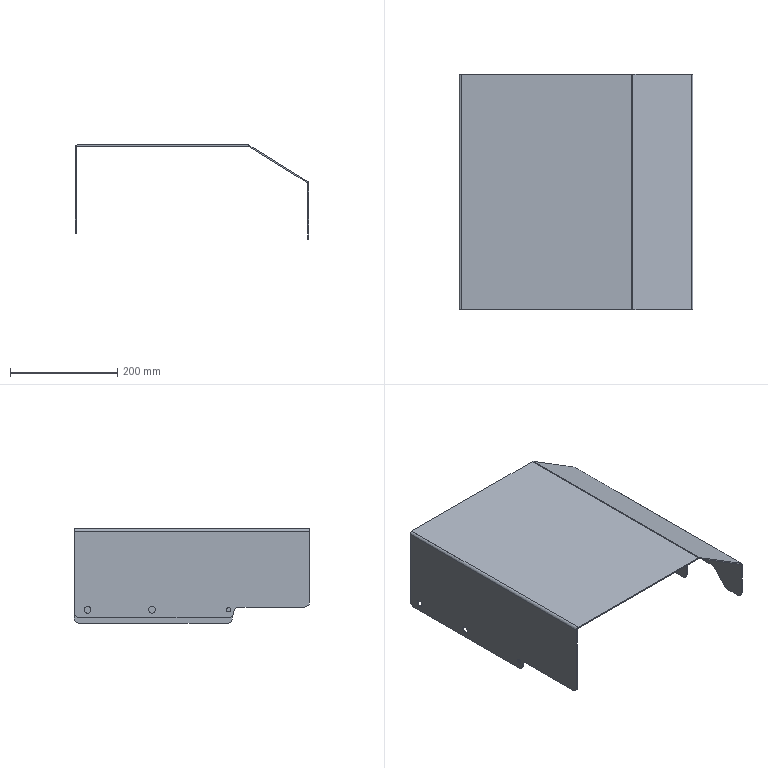Part | SolidWorks | features ICE 2, Fillet 1, FlatPattern 1, SMBaseFlange 1, SheetMetal 1 | 1 solid | 53 faces | box 436 x 439 x 176 mm | volume 705533 mm3 | plane 30 | cylinder 23 | commonest cylinder face diameters 20 x11 12.5 x4 5 x3 9.6 x3 8 x2
STEP:
#1=CARTESIAN_POINT('',(2.3,194.5,8.75));
#2=VERTEX_POINT('',#1);
#3=CARTESIAN_POINT('',(2.3,194.5,21.25));
#4=VERTEX_POINT('',#3);
#5=CARTESIAN_POINT('',(2.3,194.5,15.));
#6=DIRECTION('',(-1.,0.,0.));
#7=DIRECTION('',(0.,0.,-1.));
#8=AXIS2_PLACEMENT_3D('',#5,#6,#7);
#9=CIRCLE('',#8,6.25);
#10=EDGE_CURVE('',#2,#4,#9,.T.);
#11=ORIENTED_EDGE('',*,*,#10,.F.);
#12=CARTESIAN_POINT('',(0.,194.5,8.75));
#13=VERTEX_POINT('',#12);
#14=CARTESIAN_POINT('',(436.001,194.5,8.75));
#15=DIRECTION('',(-1.,0.,0.));
#16=VECTOR('',#15,1000.);
#17=LINE('',#14,#16);
#18=EDGE_CURVE('',#2,#13,#17,.T.);
#19=ORIENTED_EDGE('',*,*,#18,.T.);
#20=CARTESIAN_POINT('',(0.,194.5,21.25));
#21=VERTEX_POINT('',#20);
#22=CARTESIAN_POINT('',(0.,194.5,15.));
#23=DIRECTION('',(-1.,0.,0.));
#24=DIRECTION('',(0.,0.,1.));
#25=AXIS2_PLACEMENT_3D('',#22,#23,#24);
#26=CIRCLE('',#25,6.25);
#27=EDGE_CURVE('',#13,#21,#26,.T.);
#28=ORIENTED_EDGE('',*,*,#27,.T.);
#29=CARTESIAN_POINT('',(436.001,194.5,21.25));
#30=DIRECTION('',(-1.,0.,0.));
#31=VECTOR('',#30,1000.);
#32=LINE('',#29,#31);
#33=EDGE_CURVE('',#4,#21,#32,.T.);
#34=ORIENTED_EDGE('',*,*,#33,.F.);
#35=EDGE_LOOP('',(#11,#19,#28,#34));
#36=FACE_OUTER_BOUND('',#35,.T.);
#37=CARTESIAN_POINT('',(436.001,194.5,15.));
#38=DIRECTION('',(-1.,0.,0.));
#39=DIRECTION('',(0.,0.,1.));
#40=AXIS2_PLACEMENT_3D('',#37,#38,#39);
#41=CYLINDRICAL_SURFACE('',#40,6.25);
#42=ADVANCED_FACE('',(#36),#41,.F.);
#43=CARTESIAN_POINT('',(2.3,74.5,8.75));
#44=VERTEX_POINT('',#43);
#45=CARTESIAN_POINT('',(2.3,74.5,21.25));
#46=VERTEX_POINT('',#45);
#47=CARTESIAN_POINT('',(2.3,74.5,15.));
#48=DIRECTION('',(-1.,0.,0.));
#49=DIRECTION('',(0.,0.,-1.));
#50=AXIS2_PLACEMENT_3D('',#47,#48,#49);
#51=CIRCLE('',#50,6.25);
#52=EDGE_CURVE('',#44,#46,#51,.T.);
#53=ORIENTED_EDGE('',*,*,#52,.F.);
#54=CARTESIAN_POINT('',(0.,74.5,8.75));
#55=VERTEX_POINT('',#54);
#56=CARTESIAN_POINT('',(436.001,74.5,8.75));
#57=DIRECTION('',(-1.,0.,0.));
#58=VECTOR('',#57,1000.);
#59=LINE('',#56,#58);
#60=EDGE_CURVE('',#44,#55,#59,.T.);
#61=ORIENTED_EDGE('',*,*,#60,.T.);
#62=CARTESIAN_POINT('',(0.,74.5,21.25));
#63=VERTEX_POINT('',#62);
#64=CARTESIAN_POINT('',(0.,74.5,15.));
#65=DIRECTION('',(-1.,0.,0.));
#66=DIRECTION('',(0.,0.,1.));
#67=AXIS2_PLACEMENT_3D('',#64,#65,#66);
#68=CIRCLE('',#67,6.25);
#69=EDGE_CURVE('',#55,#63,#68,.T.);
#70=ORIENTED_EDGE('',*,*,#69,.T.);
#71=CARTESIAN_POINT('',(436.001,74.5,21.25));
#72=DIRECTION('',(-1.,0.,0.));
#73=VECTOR('',#72,1000.);
#74=LINE('',#71,#73);
#75=EDGE_CURVE('',#46,#63,#74,.T.);
#76=ORIENTED_EDGE('',*,*,#75,.F.);
#77=EDGE_LOOP('',(#53,#61,#70,#76));
#78=FACE_OUTER_BOUND('',#77,.T.);
#79=CARTESIAN_POINT('',(436.001,74.5,15.));
#80=DIRECTION('',(-1.,0.,0.));
#81=DIRECTION('',(0.,0.,1.));
#82=AXIS2_PLACEMENT_3D('',#79,#80,#81);
#83=CYLINDRICAL_SURFACE('',#82,6.25);
#84=ADVANCED_FACE('',(#78),#83,.F.);
#85=CARTESIAN_POINT('',(2.3,-68.5,11.));
#86=VERTEX_POINT('',#85);
#87=CARTESIAN_POINT('',(2.3,-68.5,19.));
#88=VERTEX_POINT('',#87);
#89=CARTESIAN_POINT('',(2.3,-68.5,15.));
#90=DIRECTION('',(-1.,0.,0.));
#91=DIRECTION('',(0.,0.,-1.));
#92=AXIS2_PLACEMENT_3D('',#89,#90,#91);
#93=CIRCLE('',#92,4.);
#94=EDGE_CURVE('',#86,#88,#93,.T.);
#95=ORIENTED_EDGE('',*,*,#94,.F.);
#96=CARTESIAN_POINT('',(0.,-68.5,11.));
#97=VERTEX_POINT('',#96);
#98=CARTESIAN_POINT('',(436.001,-68.5,11.));
#99=DIRECTION('',(-1.,0.,0.));
#100=VECTOR('',#99,1000.);
#101=LINE('',#98,#100);
#102=EDGE_CURVE('',#86,#97,#101,.T.);
#103=ORIENTED_EDGE('',*,*,#102,.T.);
#104=CARTESIAN_POINT('',(0.,-68.5,19.));
#105=VERTEX_POINT('',#104);
#106=CARTESIAN_POINT('',(0.,-68.5,15.));
#107=DIRECTION('',(-1.,0.,0.));
#108=DIRECTION('',(0.,0.,1.));
#109=AXIS2_PLACEMENT_3D('',#106,#107,#108);
#110=CIRCLE('',#109,4.);
#111=EDGE_CURVE('',#97,#105,#110,.T.);
#112=ORIENTED_EDGE('',*,*,#111,.T.);
#113=CARTESIAN_POINT('',(436.001,-68.5,19.));
#114=DIRECTION('',(-1.,0.,0.));
#115=VECTOR('',#114,1000.);
#116=LINE('',#113,#115);
#117=EDGE_CURVE('',#88,#105,#116,.T.);
#118=ORIENTED_EDGE('',*,*,#117,.F.);
#119=EDGE_LOOP('',(#95,#103,#112,#118));
#120=FACE_OUTER_BOUND('',#119,.T.);
#121=CARTESIAN_POINT('',(436.001,-68.5,15.));
#122=DIRECTION('',(-1.,0.,0.));
#123=DIRECTION('',(0.,0.,1.));
#124=AXIS2_PLACEMENT_3D('',#121,#122,#123);
#125=CYLINDRICAL_SURFACE('',#124,4.);
#126=ADVANCED_FACE('',(#120),#125,.F.);
#127=CARTESIAN_POINT('',(0.,219.5,161.2));
#128=VERTEX_POINT('',#127);
#129=CARTESIAN_POINT('',(2.3,219.5,161.2));
#130=VERTEX_POINT('',#129);
#131=CARTESIAN_POINT('',(0.,219.5,161.2));
#132=DIRECTION('',(1.,0.,0.));
#133=VECTOR('',#132,1000.);
#134=LINE('',#131,#133);
#135=EDGE_CURVE('',#128,#130,#134,.T.);
#136=ORIENTED_EDGE('',*,*,#135,.F.);
#137=CARTESIAN_POINT('',(4.8,219.5,166.));
#138=VERTEX_POINT('',#137);
#139=CARTESIAN_POINT('',(4.8,219.5,161.2));
#140=DIRECTION('',(0.,1.,0.));
#141=DIRECTION('',(0.,0.,-1.));
#142=AXIS2_PLACEMENT_3D('',#139,#140,#141);
#143=CIRCLE('',#142,4.8);
#144=EDGE_CURVE('',#128,#138,#143,.T.);
#145=ORIENTED_EDGE('',*,*,#144,.T.);
#146=CARTESIAN_POINT('',(4.8,219.5,163.7));
#147=VERTEX_POINT('',#146);
#148=CARTESIAN_POINT('',(4.8,219.5,163.7));
#149=DIRECTION('',(0.,0.,1.));
#150=VECTOR('',#149,1000.);
#151=LINE('',#148,#150);
#152=EDGE_CURVE('',#147,#138,#151,.T.);
#153=ORIENTED_EDGE('',*,*,#152,.F.);
#154=CARTESIAN_POINT('',(4.8,219.5,161.2));
#155=DIRECTION('',(0.,1.,0.));
#156=DIRECTION('',(1.,0.,0.));
#157=AXIS2_PLACEMENT_3D('',#154,#155,#156);
#158=CIRCLE('',#157,2.5);
#159=EDGE_CURVE('',#130,#147,#158,.T.);
#160=ORIENTED_EDGE('',*,*,#159,.F.);
#161=EDGE_LOOP('',(#136,#145,#153,#160));
#162=FACE_OUTER_BOUND('',#161,.T.);
#163=CARTESIAN_POINT('',(0.,219.5,161.2));
#164=DIRECTION('',(0.,1.,0.));
#165=DIRECTION('',(0.,0.,1.));
#166=AXIS2_PLACEMENT_3D('',#163,#164,#165);
#167=PLANE('',#166);
#168=ADVANCED_FACE('',(#162),#167,.T.);
#169=CARTESIAN_POINT('',(2.3,219.5,10.));
#170=VERTEX_POINT('',#169);
#171=CARTESIAN_POINT('',(2.3,219.5,0.));
#172=DIRECTION('',(0.,0.,1.));
#173=VECTOR('',#172,1000.);
#174=LINE('',#171,#173);
#175=EDGE_CURVE('',#170,#130,#174,.T.);
#176=ORIENTED_EDGE('',*,*,#175,.F.);
#177=CARTESIAN_POINT('',(0.,219.5,10.));
#178=VERTEX_POINT('',#177);
#179=CARTESIAN_POINT('',(4.8,219.5,10.));
#180=DIRECTION('',(-1.,0.,0.));
#181=VECTOR('',#180,1000.);
#182=LINE('',#179,#181);
#183=EDGE_CURVE('',#170,#178,#182,.T.);
#184=ORIENTED_EDGE('',*,*,#183,.T.);
#185=CARTESIAN_POINT('',(0.,219.5,0.));
#186=DIRECTION('',(0.,0.,1.));
#187=VECTOR('',#186,1000.);
#188=LINE('',#185,#187);
#189=EDGE_CURVE('',#178,#128,#188,.T.);
#190=ORIENTED_EDGE('',*,*,#189,.T.);
#191=ORIENTED_EDGE('',*,*,#135,.T.);
#192=EDGE_LOOP('',(#176,#184,#190,#191));
#193=FACE_OUTER_BOUND('',#192,.T.);
#194=CARTESIAN_POINT('',(4.8,219.5,163.7));
#195=DIRECTION('',(0.,1.,0.));
#196=DIRECTION('',(0.,0.,1.));
#197=AXIS2_PLACEMENT_3D('',#194,#195,#196);
#198=PLANE('',#197);
#199=ADVANCED_FACE('',(#193),#198,.T.);
#200=CARTESIAN_POINT('',(4.8,-219.5,166.));
#201=VERTEX_POINT('',#200);
#202=CARTESIAN_POINT('',(4.8,-219.5,163.7));
#203=VERTEX_POINT('',#202);
#204=CARTESIAN_POINT('',(4.8,-219.5,166.));
#205=DIRECTION('',(0.,0.,-1.));
#206=VECTOR('',#205,1000.);
#207=LINE('',#204,#206);
#208=EDGE_CURVE('',#201,#203,#207,.T.);
#209=ORIENTED_EDGE('',*,*,#208,.F.);
#210=CARTESIAN_POINT('',(0.,-219.5,161.2));
#211=VERTEX_POINT('',#210);
#212=CARTESIAN_POINT('',(4.8,-219.5,161.2));
#213=DIRECTION('',(0.,1.,0.));
#214=DIRECTION('',(0.,0.,-1.));
#215=AXIS2_PLACEMENT_3D('',#212,#213,#214);
#216=CIRCLE('',#215,4.8);
#217=EDGE_CURVE('',#211,#201,#216,.T.);
#218=ORIENTED_EDGE('',*,*,#217,.F.);
#219=CARTESIAN_POINT('',(2.3,-219.5,161.2));
#220=VERTEX_POINT('',#219);
#221=CARTESIAN_POINT('',(2.3,-219.5,161.2));
#222=DIRECTION('',(-1.,0.,0.));
#223=VECTOR('',#222,1000.);
#224=LINE('',#221,#223);
#225=EDGE_CURVE('',#220,#211,#224,.T.);
#226=ORIENTED_EDGE('',*,*,#225,.F.);
#227=CARTESIAN_POINT('',(4.8,-219.5,161.2));
#228=DIRECTION('',(0.,1.,0.));
#229=DIRECTION('',(1.,0.,0.));
#230=AXIS2_PLACEMENT_3D('',#227,#228,#229);
#231=CIRCLE('',#230,2.5);
#232=EDGE_CURVE('',#220,#203,#231,.T.);
#233=ORIENTED_EDGE('',*,*,#232,.T.);
#234=EDGE_LOOP('',(#209,#218,#226,#233));
#235=FACE_OUTER_BOUND('',#234,.T.);
#236=CARTESIAN_POINT('',(4.8,-219.5,166.));
#237=DIRECTION('',(0.,-1.,0.));
#238=DIRECTION('',(0.,0.,-1.));
#239=AXIS2_PLACEMENT_3D('',#236,#237,#238);
#240=PLANE('',#239);
#241=ADVANCED_FACE('',(#235),#240,.T.);
#242=CARTESIAN_POINT('',(321.634,-219.5,166.));
#243=VERTEX_POINT('',#242);
#244=CARTESIAN_POINT('',(0.,-219.5,166.));
#245=DIRECTION('',(1.,0.,0.));
#246=VECTOR('',#245,1000.);
#247=LINE('',#244,#246);
#248=EDGE_CURVE('',#201,#243,#247,.T.);
#249=ORIENTED_EDGE('',*,*,#248,.F.);
#250=ORIENTED_EDGE('',*,*,#208,.T.);
#251=CARTESIAN_POINT('',(321.634,-219.5,163.7));
#252=VERTEX_POINT('',#251);
#253=CARTESIAN_POINT('',(0.,-219.5,163.7));
#254=DIRECTION('',(1.,0.,0.));
#255=VECTOR('',#254,1000.);
#256=LINE('',#253,#255);
#257=EDGE_CURVE('',#203,#252,#256,.T.);
#258=ORIENTED_EDGE('',*,*,#257,.T.);
#259=CARTESIAN_POINT('',(321.634,-219.5,163.7));
#260=DIRECTION('',(0.,0.,1.));
#261=VECTOR('',#260,1000.);
#262=LINE('',#259,#261);
#263=EDGE_CURVE('',#252,#243,#262,.T.);
#264=ORIENTED_EDGE('',*,*,#263,.T.);
#265=EDGE_LOOP('',(#249,#250,#258,#264));
#266=FACE_OUTER_BOUND('',#265,.T.);
#267=CARTESIAN_POINT('',(2.3,-219.5,161.2));
#268=DIRECTION('',(0.,-1.,0.));
#269=DIRECTION('',(0.,0.,-1.));
#270=AXIS2_PLACEMENT_3D('',#267,#268,#269);
#271=PLANE('',#270);
#272=ADVANCED_FACE('',(#266),#271,.T.);
#273=CARTESIAN_POINT('',(321.634,219.5,166.));
#274=VERTEX_POINT('',#273);
#275=CARTESIAN_POINT('',(321.634,219.5,163.7));
#276=VERTEX_POINT('',#275);
#277=CARTESIAN_POINT('',(321.634,219.5,166.));
#278=DIRECTION('',(0.,0.,-1.));
#279=VECTOR('',#278,1000.);
#280=LINE('',#277,#279);
#281=EDGE_CURVE('',#274,#276,#280,.T.);
#282=ORIENTED_EDGE('',*,*,#281,.F.);
#283=CARTESIAN_POINT('',(324.161,219.5,165.281));
#284=VERTEX_POINT('',#283);
#285=CARTESIAN_POINT('',(321.634,219.5,161.2));
#286=DIRECTION('',(0.,1.,0.));
#287=DIRECTION('',(0.,0.,-1.));
#288=AXIS2_PLACEMENT_3D('',#285,#286,#287);
#289=CIRCLE('',#288,4.8);
#290=EDGE_CURVE('',#274,#284,#289,.T.);
#291=ORIENTED_EDGE('',*,*,#290,.T.);
#292=CARTESIAN_POINT('',(322.95,219.5,163.325));
#293=VERTEX_POINT('',#292);
#294=CARTESIAN_POINT('',(322.95,219.5,163.325));
#295=DIRECTION('',(0.5266,0.,0.8501));
#296=VECTOR('',#295,1000.);
#297=LINE('',#294,#296);
#298=EDGE_CURVE('',#293,#284,#297,.T.);
#299=ORIENTED_EDGE('',*,*,#298,.F.);
#300=CARTESIAN_POINT('',(321.634,219.5,161.2));
#301=DIRECTION('',(0.,1.,0.));
#302=DIRECTION('',(1.,0.,0.));
#303=AXIS2_PLACEMENT_3D('',#300,#301,#302);
#304=CIRCLE('',#303,2.5);
#305=EDGE_CURVE('',#276,#293,#304,.T.);
#306=ORIENTED_EDGE('',*,*,#305,.F.);
#307=EDGE_LOOP('',(#282,#291,#299,#306));
#308=FACE_OUTER_BOUND('',#307,.T.);
#309=CARTESIAN_POINT('',(321.634,219.5,166.));
#310=DIRECTION('',(0.,1.,0.));
#311=DIRECTION('',(0.,0.,1.));
#312=AXIS2_PLACEMENT_3D('',#309,#310,#311);
#313=PLANE('',#312);
#314=ADVANCED_FACE('',(#308),#313,.T.);
#315=CARTESIAN_POINT('',(0.,219.5,166.));
#316=DIRECTION('',(1.,0.,0.));
#317=VECTOR('',#316,1000.);
#318=LINE('',#315,#317);
#319=EDGE_CURVE('',#138,#274,#318,.T.);
#320=ORIENTED_EDGE('',*,*,#319,.T.);
#321=ORIENTED_EDGE('',*,*,#281,.T.);
#322=CARTESIAN_POINT('',(0.,219.5,163.7));
#323=DIRECTION('',(1.,0.,0.));
#324=VECTOR('',#323,1000.);
#325=LINE('',#322,#324);
#326=EDGE_CURVE('',#147,#276,#325,.T.);
#327=ORIENTED_EDGE('',*,*,#326,.F.);
#328=ORIENTED_EDGE('',*,*,#152,.T.);
#329=EDGE_LOOP('',(#320,#321,#327,#328));
#330=FACE_OUTER_BOUND('',#329,.T.);
#331=CARTESIAN_POINT('',(322.95,219.5,163.325));
#332=DIRECTION('',(0.,1.,0.));
#333=DIRECTION('',(0.,0.,1.));
#334=AXIS2_PLACEMENT_3D('',#331,#332,#333);
#335=PLANE('',#334);
#336=ADVANCED_FACE('',(#330),#335,.T.);
#337=CARTESIAN_POINT('',(324.161,-219.5,165.281));
#338=VERTEX_POINT('',#337);
#339=CARTESIAN_POINT('',(322.95,-219.5,163.325));
#340=VERTEX_POINT('',#339);
#341=CARTESIAN_POINT('',(324.161,-219.5,165.281));
#342=DIRECTION('',(-0.5266,0.,-0.8501));
#343=VECTOR('',#342,1000.);
#344=LINE('',#341,#343);
#345=EDGE_CURVE('',#338,#340,#344,.T.);
#346=ORIENTED_EDGE('',*,*,#345,.F.);
#347=CARTESIAN_POINT('',(321.634,-219.5,161.2));
#348=DIRECTION('',(0.,1.,0.));
#349=DIRECTION('',(0.,0.,-1.));
#350=AXIS2_PLACEMENT_3D('',#347,#348,#349);
#351=CIRCLE('',#350,4.8);
#352=EDGE_CURVE('',#243,#338,#351,.T.);
#353=ORIENTED_EDGE('',*,*,#352,.F.);
#354=ORIENTED_EDGE('',*,*,#263,.F.);
#355=CARTESIAN_POINT('',(321.634,-219.5,161.2));
#356=DIRECTION('',(0.,1.,0.));
#357=DIRECTION('',(1.,0.,0.));
#358=AXIS2_PLACEMENT_3D('',#355,#356,#357);
#359=CIRCLE('',#358,2.5);
#360=EDGE_CURVE('',#252,#340,#359,.T.);
#361=ORIENTED_EDGE('',*,*,#360,.T.);
#362=EDGE_LOOP('',(#346,#353,#354,#361));
#363=FACE_OUTER_BOUND('',#362,.T.);
#364=CARTESIAN_POINT('',(324.161,-219.5,165.281));
#365=DIRECTION('',(0.,-1.,0.));
#366=DIRECTION('',(0.,0.,-1.));
#367=AXIS2_PLACEMENT_3D('',#364,#365,#366);
#368=PLANE('',#367);
#369=ADVANCED_FACE('',(#363),#368,.T.);
#370=CARTESIAN_POINT('',(433.728,-219.5,97.408));
#371=VERTEX_POINT('',#370);
#372=CARTESIAN_POINT('',(323.,-219.5,166.));
#373=DIRECTION('',(0.8501,0.,-0.5266));
#374=VECTOR('',#373,1000.);
#375=LINE('',#372,#374);
#376=EDGE_CURVE('',#338,#371,#375,.T.);
#377=ORIENTED_EDGE('',*,*,#376,.F.);
#378=ORIENTED_EDGE('',*,*,#345,.T.);
#379=CARTESIAN_POINT('',(432.517,-219.5,95.452));
#380=VERTEX_POINT('',#379);
#381=CARTESIAN_POINT('',(321.789,-219.5,164.045));
#382=DIRECTION('',(0.8501,0.,-0.5266));
#383=VECTOR('',#382,1000.);
#384=LINE('',#381,#383);
#385=EDGE_CURVE('',#340,#380,#384,.T.);
#386=ORIENTED_EDGE('',*,*,#385,.T.);
#387=CARTESIAN_POINT('',(432.517,-219.5,95.452));
#388=DIRECTION('',(0.5266,0.,0.8501));
#389=VECTOR('',#388,1000.);
#390=LINE('',#387,#389);
#391=EDGE_CURVE('',#380,#371,#390,.T.);
#392=ORIENTED_EDGE('',*,*,#391,.T.);
#393=EDGE_LOOP('',(#377,#378,#386,#392));
#394=FACE_OUTER_BOUND('',#393,.T.);
#395=CARTESIAN_POINT('',(321.634,-219.5,163.7));
#396=DIRECTION('',(0.,-1.,0.));
#397=DIRECTION('',(0.,0.,-1.));
#398=AXIS2_PLACEMENT_3D('',#395,#396,#397);
#399=PLANE('',#398);
#400=ADVANCED_FACE('',(#394),#399,.T.);
#401=CARTESIAN_POINT('',(433.728,219.5,97.408));
#402=VERTEX_POINT('',#401);
#403=CARTESIAN_POINT('',(432.517,219.5,95.452));
#404=VERTEX_POINT('',#403);
#405=CARTESIAN_POINT('',(433.728,219.5,97.408));
#406=DIRECTION('',(-0.5266,0.,-0.8501));
#407=VECTOR('',#406,1000.);
#408=LINE('',#405,#407);
#409=EDGE_CURVE('',#402,#404,#408,.T.);
#410=ORIENTED_EDGE('',*,*,#409,.F.);
#411=CARTESIAN_POINT('',(436.,219.5,93.327));
#412=VERTEX_POINT('',#411);
#413=CARTESIAN_POINT('',(431.2,219.5,93.327));
#414=DIRECTION('',(0.,1.,0.));
#415=DIRECTION('',(0.,0.,-1.));
#416=AXIS2_PLACEMENT_3D('',#413,#414,#415);
#417=CIRCLE('',#416,4.8);
#418=EDGE_CURVE('',#402,#412,#417,.T.);
#419=ORIENTED_EDGE('',*,*,#418,.T.);
#420=CARTESIAN_POINT('',(433.7,219.5,93.327));
#421=VERTEX_POINT('',#420);
#422=CARTESIAN_POINT('',(433.7,219.5,93.327));
#423=DIRECTION('',(1.,0.,0.));
#424=VECTOR('',#423,1000.);
#425=LINE('',#422,#424);
#426=EDGE_CURVE('',#421,#412,#425,.T.);
#427=ORIENTED_EDGE('',*,*,#426,.F.);
#428=CARTESIAN_POINT('',(431.2,219.5,93.327));
#429=DIRECTION('',(0.,1.,0.));
#430=DIRECTION('',(1.,0.,0.));
#431=AXIS2_PLACEMENT_3D('',#428,#429,#430);
#432=CIRCLE('',#431,2.5);
#433=EDGE_CURVE('',#404,#421,#432,.T.);
#434=ORIENTED_EDGE('',*,*,#433,.F.);
#435=EDGE_LOOP('',(#410,#419,#427,#434));
#436=FACE_OUTER_BOUND('',#435,.T.);
#437=CARTESIAN_POINT('',(433.728,219.5,97.408));
#438=DIRECTION('',(0.,1.,0.));
#439=DIRECTION('',(0.,0.,1.));
#440=AXIS2_PLACEMENT_3D('',#437,#438,#439);
#441=PLANE('',#440);
#442=ADVANCED_FACE('',(#436),#441,.T.);
#443=CARTESIAN_POINT('',(323.,219.5,166.));
#444=DIRECTION('',(0.8501,0.,-0.5266));
#445=VECTOR('',#444,1000.);
#446=LINE('',#443,#445);
#447=EDGE_CURVE('',#284,#402,#446,.T.);
#448=ORIENTED_EDGE('',*,*,#447,.T.);
#449=ORIENTED_EDGE('',*,*,#409,.T.);
#450=CARTESIAN_POINT('',(321.789,219.5,164.045));
#451=DIRECTION('',(0.8501,0.,-0.5266));
#452=VECTOR('',#451,1000.);
#453=LINE('',#450,#452);
#454=EDGE_CURVE('',#293,#404,#453,.T.);
#455=ORIENTED_EDGE('',*,*,#454,.F.);
#456=ORIENTED_EDGE('',*,*,#298,.T.);
#457=EDGE_LOOP('',(#448,#449,#455,#456));
#458=FACE_OUTER_BOUND('',#457,.T.);
#459=CARTESIAN_POINT('',(433.7,219.5,93.327));
#460=DIRECTION('',(0.,1.,0.));
#461=DIRECTION('',(0.,0.,1.));
#462=AXIS2_PLACEMENT_3D('',#459,#460,#461);
#463=PLANE('',#462);
#464=ADVANCED_FACE('',(#458),#463,.T.);
#465=CARTESIAN_POINT('',(436.,-219.5,93.327));
#466=VERTEX_POINT('',#465);
#467=CARTESIAN_POINT('',(433.7,-219.5,93.327));
#468=VERTEX_POINT('',#467);
#469=CARTESIAN_POINT('',(436.,-219.5,93.327));
#470=DIRECTION('',(-1.,0.,0.));
#471=VECTOR('',#470,1000.);
#472=LINE('',#469,#471);
#473=EDGE_CURVE('',#466,#468,#472,.T.);
#474=ORIENTED_EDGE('',*,*,#473,.F.);
#475=CARTESIAN_POINT('',(431.2,-219.5,93.327));
#476=DIRECTION('',(0.,1.,0.));
#477=DIRECTION('',(0.,0.,-1.));
#478=AXIS2_PLACEMENT_3D('',#475,#476,#477);
#479=CIRCLE('',#478,4.8);
#480=EDGE_CURVE('',#371,#466,#479,.T.);
#481=ORIENTED_EDGE('',*,*,#480,.F.);
#482=ORIENTED_EDGE('',*,*,#391,.F.);
#483=CARTESIAN_POINT('',(431.2,-219.5,93.327));
#484=DIRECTION('',(0.,1.,0.));
#485=DIRECTION('',(1.,0.,0.));
#486=AXIS2_PLACEMENT_3D('',#483,#484,#485);
#487=CIRCLE('',#486,2.5);
#488=EDGE_CURVE('',#380,#468,#487,.T.);
#489=ORIENTED_EDGE('',*,*,#488,.T.);
#490=EDGE_LOOP('',(#474,#481,#482,#489));
#491=FACE_OUTER_BOUND('',#490,.T.);
#492=CARTESIAN_POINT('',(436.,-219.5,93.327));
#493=DIRECTION('',(0.,-1.,0.));
#494=DIRECTION('',(0.,0.,-1.));
#495=AXIS2_PLACEMENT_3D('',#492,#493,#494);
#496=PLANE('',#495);
#497=ADVANCED_FACE('',(#491),#496,.T.);
#498=CARTESIAN_POINT('',(433.7,-219.5,30.));
#499=VERTEX_POINT('',#498);
#500=CARTESIAN_POINT('',(433.7,-219.5,96.));
#501=DIRECTION('',(0.,0.,-1.));
#502=VECTOR('',#501,1000.);
#503=LINE('',#500,#502);
#504=EDGE_CURVE('',#468,#499,#503,.T.);
#505=ORIENTED_EDGE('',*,*,#504,.T.);
#506=CARTESIAN_POINT('',(436.,-219.5,30.));
#507=VERTEX_POINT('',#506);
#508=CARTESIAN_POINT('',(436.,-219.5,30.));
#509=DIRECTION('',(1.,0.,0.));
#510=VECTOR('',#509,1000.);
#511=LINE('',#508,#510);
#512=EDGE_CURVE('',#499,#507,#511,.T.);
#513=ORIENTED_EDGE('',*,*,#512,.T.);
#514=CARTESIAN_POINT('',(436.,-219.5,96.));
#515=DIRECTION('',(0.,0.,-1.));
#516=VECTOR('',#515,1000.);
#517=LINE('',#514,#516);
#518=EDGE_CURVE('',#466,#507,#517,.T.);
#519=ORIENTED_EDGE('',*,*,#518,.F.);
#520=ORIENTED_EDGE('',*,*,#473,.T.);
#521=EDGE_LOOP('',(#505,#513,#519,#520));
#522=FACE_OUTER_BOUND('',#521,.T.);
#523=CARTESIAN_POINT('',(432.517,-219.5,95.452));
#524=DIRECTION('',(0.,-1.,0.));
#525=DIRECTION('',(0.,0.,-1.));
#526=AXIS2_PLACEMENT_3D('',#523,#524,#525);
#527=PLANE('',#526);
#528=ADVANCED_FACE('',(#522),#527,.T.);
#529=CARTESIAN_POINT('',(436.,209.5,-10.));
#530=VERTEX_POINT('',#529);
#531=CARTESIAN_POINT('',(436.,-65.5,-10.));
#532=VERTEX_POINT('',#531);
#533=CARTESIAN_POINT('',(436.,219.5,-10.));
#534=DIRECTION('',(0.,-1.,0.));
#535=VECTOR('',#534,1000.);
#536=LINE('',#533,#535);
#537=EDGE_CURVE('',#530,#532,#536,.T.);
#538=ORIENTED_EDGE('',*,*,#537,.F.);
#539=CARTESIAN_POINT('',(436.,219.5,0.));
#540=VERTEX_POINT('',#539);
#541=CARTESIAN_POINT('',(436.,209.5,0.));
#542=DIRECTION('',(1.,0.,0.));
#543=DIRECTION('',(0.,0.,1.));
#544=AXIS2_PLACEMENT_3D('',#541,#542,#543);
#545=CIRCLE('',#544,10.);
#546=EDGE_CURVE('',#530,#540,#545,.T.);
#547=ORIENTED_EDGE('',*,*,#546,.T.);
#548=CARTESIAN_POINT('',(436.,219.5,96.));
#549=DIRECTION('',(0.,0.,-1.));
#550=VECTOR('',#549,1000.);
#551=LINE('',#548,#550);
#552=EDGE_CURVE('',#412,#540,#551,.T.);
#553=ORIENTED_EDGE('',*,*,#552,.F.);
#554=CARTESIAN_POINT('',(436.,219.5,93.327));
#555=DIRECTION('',(0.,-1.,0.));
#556=VECTOR('',#555,1000.);
#557=LINE('',#554,#556);
#558=EDGE_CURVE('',#412,#466,#557,.T.);
#559=ORIENTED_EDGE('',*,*,#558,.T.);
#560=ORIENTED_EDGE('',*,*,#518,.T.);
#561=CARTESIAN_POINT('',(436.,-209.5,20.));
#562=VERTEX_POINT('',#561);
#563=CARTESIAN_POINT('',(436.,-209.5,30.));
#564=DIRECTION('',(1.,0.,0.));
#565=DIRECTION('',(0.,0.,1.));
#566=AXIS2_PLACEMENT_3D('',#563,#564,#565);
#567=CIRCLE('',#566,10.);
#568=EDGE_CURVE('',#507,#562,#567,.T.);
#569=ORIENTED_EDGE('',*,*,#568,.T.);
#570=CARTESIAN_POINT('',(436.,-183.907,20.));
#571=VERTEX_POINT('',#570);
#572=CARTESIAN_POINT('',(436.,-179.5,20.));
#573=DIRECTION('',(0.,-1.,0.));
#574=VECTOR('',#573,1000.);
#575=LINE('',#572,#574);
#576=EDGE_CURVE('',#571,#562,#575,.T.);
#577=ORIENTED_EDGE('',*,*,#576,.F.);
#578=CARTESIAN_POINT('',(436.,-176.526,23.252));
#579=VERTEX_POINT('',#578);
#580=CARTESIAN_POINT('',(436.,-183.907,30.));
#581=DIRECTION('',(1.,0.,0.));
#582=DIRECTION('',(0.,0.,1.));
#583=AXIS2_PLACEMENT_3D('',#580,#581,#582);
#584=CIRCLE('',#583,10.);
#585=EDGE_CURVE('',#571,#579,#584,.T.);
#586=ORIENTED_EDGE('',*,*,#585,.T.);
#587=CARTESIAN_POINT('',(436.,-150.474,51.748));
#588=VERTEX_POINT('',#587);
#589=CARTESIAN_POINT('',(436.,-147.5,55.));
#590=DIRECTION('',(0.,-0.6748,-0.738));
#591=VECTOR('',#590,1000.);
#592=LINE('',#589,#591);
#593=EDGE_CURVE('',#588,#579,#592,.T.);
#594=ORIENTED_EDGE('',*,*,#593,.F.);
#595=CARTESIAN_POINT('',(436.,-143.093,55.));
#596=VERTEX_POINT('',#595);
#597=CARTESIAN_POINT('',(436.,-143.093,45.));
#598=DIRECTION('',(-1.,0.,0.));
#599=DIRECTION('',(0.,0.,1.));
#600=AXIS2_PLACEMENT_3D('',#597,#598,#599);
#601=CIRCLE('',#600,10.);
#602=EDGE_CURVE('',#588,#596,#601,.T.);
#603=ORIENTED_EDGE('',*,*,#602,.T.);
#604=CARTESIAN_POINT('',(436.,-111.907,55.));
#605=VERTEX_POINT('',#604);
#606=CARTESIAN_POINT('',(436.,-107.5,55.));
#607=DIRECTION('',(0.,-1.,0.));
#608=VECTOR('',#607,1000.);
#609=LINE('',#606,#608);
#610=EDGE_CURVE('',#605,#596,#609,.T.);
#611=ORIENTED_EDGE('',*,*,#610,.F.);
#612=CARTESIAN_POINT('',(436.,-104.526,51.748));
#613=VERTEX_POINT('',#612);
#614=CARTESIAN_POINT('',(436.,-111.907,45.));
#615=DIRECTION('',(-1.,0.,0.));
#616=DIRECTION('',(0.,0.,1.));
#617=AXIS2_PLACEMENT_3D('',#614,#615,#616);
#618=CIRCLE('',#617,10.);
#619=EDGE_CURVE('',#605,#613,#618,.T.);
#620=ORIENTED_EDGE('',*,*,#619,.T.);
#621=CARTESIAN_POINT('',(436.,-78.12,22.865));
#622=VERTEX_POINT('',#621);
#623=CARTESIAN_POINT('',(436.,-107.5,55.));
#624=DIRECTION('',(0.,-0.6748,0.738));
#625=VECTOR('',#624,1000.);
#626=LINE('',#623,#625);
#627=EDGE_CURVE('',#622,#613,#626,.T.);
#628=ORIENTED_EDGE('',*,*,#627,.F.);
#629=CARTESIAN_POINT('',(436.,-75.5,16.118));
#630=VERTEX_POINT('',#629);
#631=CARTESIAN_POINT('',(436.,-85.5,16.118));
#632=DIRECTION('',(-1.,0.,0.));
#633=DIRECTION('',(0.,0.,1.));
#634=AXIS2_PLACEMENT_3D('',#631,#632,#633);
#635=CIRCLE('',#634,10.);
#636=EDGE_CURVE('',#622,#630,#635,.T.);
#637=ORIENTED_EDGE('',*,*,#636,.T.);
#638=CARTESIAN_POINT('',(436.,-75.5,0.));
#639=VERTEX_POINT('',#638);
#640=CARTESIAN_POINT('',(436.,-75.5,-10.));
#641=DIRECTION('',(0.,0.,1.));
#642=VECTOR('',#641,1000.);
#643=LINE('',#640,#642);
#644=EDGE_CURVE('',#639,#630,#643,.T.);
#645=ORIENTED_EDGE('',*,*,#644,.F.);
#646=CARTESIAN_POINT('',(436.,-65.5,0.));
#647=DIRECTION('',(1.,0.,0.));
#648=DIRECTION('',(0.,0.,1.));
#649=AXIS2_PLACEMENT_3D('',#646,#647,#648);
#650=CIRCLE('',#649,10.);
#651=EDGE_CURVE('',#639,#532,#650,.T.);
#652=ORIENTED_EDGE('',*,*,#651,.T.);
#653=EDGE_LOOP('',(#538,#547,#553,#559,#560,#569,#577,#586,#594,#603,#611,#620,#628,#637,#645,#652));
#654=FACE_OUTER_BOUND('',#653,.T.);
#655=CARTESIAN_POINT('',(436.,219.5,96.));
#656=DIRECTION('',(-1.,0.,0.));
#657=DIRECTION('',(0.,0.,1.));
#658=AXIS2_PLACEMENT_3D('',#655,#656,#657);
#659=PLANE('',#658);
#660=ADVANCED_FACE('',(#654),#659,.F.);
#661=CARTESIAN_POINT('',(433.7,209.5,-10.));
#662=VERTEX_POINT('',#661);
#663=CARTESIAN_POINT('',(433.7,-65.5,-10.));
#664=VERTEX_POINT('',#663);
#665=CARTESIAN_POINT('',(433.7,219.5,-10.));
#666=DIRECTION('',(0.,-1.,0.));
#667=VECTOR('',#666,1000.);
#668=LINE('',#665,#667);
#669=EDGE_CURVE('',#662,#664,#668,.T.);
#670=ORIENTED_EDGE('',*,*,#669,.F.);
#671=CARTESIAN_POINT('',(433.7,209.5,-10.));
#672=DIRECTION('',(1.,0.,0.));
#673=VECTOR('',#672,1000.);
#674=LINE('',#671,#673);
#675=EDGE_CURVE('',#662,#530,#674,.T.);
#676=ORIENTED_EDGE('',*,*,#675,.T.);
#677=ORIENTED_EDGE('',*,*,#537,.T.);
#678=CARTESIAN_POINT('',(433.7,-65.5,-10.));
#679=DIRECTION('',(-1.,0.,0.));
#680=VECTOR('',#679,1000.);
#681=LINE('',#678,#680);
#682=EDGE_CURVE('',#532,#664,#681,.T.);
#683=ORIENTED_EDGE('',*,*,#682,.T.);
#684=EDGE_LOOP('',(#670,#676,#677,#683));
#685=FACE_OUTER_BOUND('',#684,.T.);
#686=CARTESIAN_POINT('',(433.7,219.5,-10.));
#687=DIRECTION('',(0.,0.,-1.));
#688=DIRECTION('',(-1.,0.,0.));
#689=AXIS2_PLACEMENT_3D('',#686,#687,#688);
#690=PLANE('',#689);
#691=ADVANCED_FACE('',(#685),#690,.T.);
#692=CARTESIAN_POINT('',(433.7,219.5,0.));
#693=VERTEX_POINT('',#692);
#694=CARTESIAN_POINT('',(433.7,219.5,96.));
#695=DIRECTION('',(0.,0.,-1.));
#696=VECTOR('',#695,1000.);
#697=LINE('',#694,#696);
#698=EDGE_CURVE('',#421,#693,#697,.T.);
#699=ORIENTED_EDGE('',*,*,#698,.T.);
#700=CARTESIAN_POINT('',(433.7,209.5,0.));
#701=DIRECTION('',(-1.,0.,0.));
#702=DIRECTION('',(0.,0.,1.));
#703=AXIS2_PLACEMENT_3D('',#700,#701,#702);
#704=CIRCLE('',#703,10.);
#705=EDGE_CURVE('',#693,#662,#704,.T.);
#706=ORIENTED_EDGE('',*,*,#705,.T.);
#707=ORIENTED_EDGE('',*,*,#669,.T.);
#708=CARTESIAN_POINT('',(433.7,-75.5,0.));
#709=VERTEX_POINT('',#708);
#710=CARTESIAN_POINT('',(433.7,-65.5,0.));
#711=DIRECTION('',(-1.,0.,0.));
#712=DIRECTION('',(0.,0.,1.));
#713=AXIS2_PLACEMENT_3D('',#710,#711,#712);
#714=CIRCLE('',#713,10.);
#715=EDGE_CURVE('',#664,#709,#714,.T.);
#716=ORIENTED_EDGE('',*,*,#715,.T.);
#717=CARTESIAN_POINT('',(433.7,-75.5,16.118));
#718=VERTEX_POINT('',#717);
#719=CARTESIAN_POINT('',(433.7,-75.5,-10.));
#720=DIRECTION('',(0.,0.,1.));
#721=VECTOR('',#720,1000.);
#722=LINE('',#719,#721);
#723=EDGE_CURVE('',#709,#718,#722,.T.);
#724=ORIENTED_EDGE('',*,*,#723,.T.);
#725=CARTESIAN_POINT('',(433.7,-78.12,22.865));
#726=VERTEX_POINT('',#725);
#727=CARTESIAN_POINT('',(433.7,-85.5,16.118));
#728=DIRECTION('',(1.,0.,0.));
#729=DIRECTION('',(0.,0.,1.));
#730=AXIS2_PLACEMENT_3D('',#727,#728,#729);
#731=CIRCLE('',#730,10.);
#732=EDGE_CURVE('',#718,#726,#731,.T.);
#733=ORIENTED_EDGE('',*,*,#732,.T.);
#734=CARTESIAN_POINT('',(433.7,-104.526,51.748));
#735=VERTEX_POINT('',#734);
#736=CARTESIAN_POINT('',(433.7,-107.5,55.));
#737=DIRECTION('',(0.,-0.6748,0.738));
#738=VECTOR('',#737,1000.);
#739=LINE('',#736,#738);
#740=EDGE_CURVE('',#726,#735,#739,.T.);
#741=ORIENTED_EDGE('',*,*,#740,.T.);
#742=CARTESIAN_POINT('',(433.7,-111.907,55.));
#743=VERTEX_POINT('',#742);
#744=CARTESIAN_POINT('',(433.7,-111.907,45.));
#745=DIRECTION('',(1.,0.,0.));
#746=DIRECTION('',(0.,0.,1.));
#747=AXIS2_PLACEMENT_3D('',#744,#745,#746);
#748=CIRCLE('',#747,10.);
#749=EDGE_CURVE('',#735,#743,#748,.T.);
#750=ORIENTED_EDGE('',*,*,#749,.T.);
#751=CARTESIAN_POINT('',(433.7,-143.093,55.));
#752=VERTEX_POINT('',#751);
#753=CARTESIAN_POINT('',(433.7,-107.5,55.));
#754=DIRECTION('',(0.,-1.,0.));
#755=VECTOR('',#754,1000.);
#756=LINE('',#753,#755);
#757=EDGE_CURVE('',#743,#752,#756,.T.);
#758=ORIENTED_EDGE('',*,*,#757,.T.);
#759=CARTESIAN_POINT('',(433.7,-150.474,51.748));
#760=VERTEX_POINT('',#759);
#761=CARTESIAN_POINT('',(433.7,-143.093,45.));
#762=DIRECTION('',(1.,0.,0.));
#763=DIRECTION('',(0.,0.,1.));
#764=AXIS2_PLACEMENT_3D('',#761,#762,#763);
#765=CIRCLE('',#764,10.);
#766=EDGE_CURVE('',#752,#760,#765,.T.);
#767=ORIENTED_EDGE('',*,*,#766,.T.);
#768=CARTESIAN_POINT('',(433.7,-176.526,23.252));
#769=VERTEX_POINT('',#768);
#770=CARTESIAN_POINT('',(433.7,-147.5,55.));
#771=DIRECTION('',(0.,-0.6748,-0.738));
#772=VECTOR('',#771,1000.);
#773=LINE('',#770,#772);
#774=EDGE_CURVE('',#760,#769,#773,.T.);
#775=ORIENTED_EDGE('',*,*,#774,.T.);
#776=CARTESIAN_POINT('',(433.7,-183.907,20.));
#777=VERTEX_POINT('',#776);
#778=CARTESIAN_POINT('',(433.7,-183.907,30.));
#779=DIRECTION('',(-1.,0.,0.));
#780=DIRECTION('',(0.,0.,1.));
#781=AXIS2_PLACEMENT_3D('',#778,#779,#780);
#782=CIRCLE('',#781,10.);
#783=EDGE_CURVE('',#769,#777,#782,.T.);
#784=ORIENTED_EDGE('',*,*,#783,.T.);
#785=CARTESIAN_POINT('',(433.7,-209.5,20.));
#786=VERTEX_POINT('',#785);
#787=CARTESIAN_POINT('',(433.7,-179.5,20.));
#788=DIRECTION('',(0.,-1.,0.));
#789=VECTOR('',#788,1000.);
#790=LINE('',#787,#789);
#791=EDGE_CURVE('',#777,#786,#790,.T.);
#792=ORIENTED_EDGE('',*,*,#791,.T.);
#793=CARTESIAN_POINT('',(433.7,-209.5,30.));
#794=DIRECTION('',(-1.,0.,0.));
#795=DIRECTION('',(0.,0.,1.));
#796=AXIS2_PLACEMENT_3D('',#793,#794,#795);
#797=CIRCLE('',#796,10.);
#798=EDGE_CURVE('',#786,#499,#797,.T.);
#799=ORIENTED_EDGE('',*,*,#798,.T.);
#800=ORIENTED_EDGE('',*,*,#504,.F.);
#801=CARTESIAN_POINT('',(433.7,219.5,93.327));
#802=DIRECTION('',(0.,-1.,0.));
#803=VECTOR('',#802,1000.);
#804=LINE('',#801,#803);
#805=EDGE_CURVE('',#421,#468,#804,.T.);
#806=ORIENTED_EDGE('',*,*,#805,.F.);
#807=EDGE_LOOP('',(#699,#706,#707,#716,#724,#733,#741,#750,#758,#767,#775,#784,#792,#799,#800,#806));
#808=FACE_OUTER_BOUND('',#807,.T.);
#809=CARTESIAN_POINT('',(433.7,219.5,96.));
#810=DIRECTION('',(-1.,0.,0.));
#811=DIRECTION('',(0.,0.,1.));
#812=AXIS2_PLACEMENT_3D('',#809,#810,#811);
#813=PLANE('',#812);
#814=ADVANCED_FACE('',(#808),#813,.T.);
#815=ORIENTED_EDGE('',*,*,#488,.F.);
#816=CARTESIAN_POINT('',(432.517,219.5,95.452));
#817=DIRECTION('',(0.,-1.,0.));
#818=VECTOR('',#817,1000.);
#819=LINE('',#816,#818);
#820=EDGE_CURVE('',#404,#380,#819,.T.);
#821=ORIENTED_EDGE('',*,*,#820,.F.);
#822=ORIENTED_EDGE('',*,*,#433,.T.);
#823=ORIENTED_EDGE('',*,*,#805,.T.);
#824=EDGE_LOOP('',(#815,#821,#822,#823));
#825=FACE_OUTER_BOUND('',#824,.T.);
#826=CARTESIAN_POINT('',(431.2,219.5,93.327));
#827=DIRECTION('',(0.,-1.,0.));
#828=DIRECTION('',(0.,0.,-1.));
#829=AXIS2_PLACEMENT_3D('',#826,#827,#828);
#830=CYLINDRICAL_SURFACE('',#829,2.5);
#831=ADVANCED_FACE('',(#825),#830,.F.);
#832=ORIENTED_EDGE('',*,*,#385,.F.);
#833=CARTESIAN_POINT('',(322.95,219.5,163.325));
#834=DIRECTION('',(0.,-1.,0.));
#835=VECTOR('',#834,1000.);
#836=LINE('',#833,#835);
#837=EDGE_CURVE('',#293,#340,#836,.T.);
#838=ORIENTED_EDGE('',*,*,#837,.F.);
#839=ORIENTED_EDGE('',*,*,#454,.T.);
#840=ORIENTED_EDGE('',*,*,#820,.T.);
#841=EDGE_LOOP('',(#832,#838,#839,#840));
#842=FACE_OUTER_BOUND('',#841,.T.);
#843=CARTESIAN_POINT('',(321.789,219.5,164.045));
#844=DIRECTION('',(-0.5266,0.,-0.8501));
#845=DIRECTION('',(-0.8501,0.,0.5266));
#846=AXIS2_PLACEMENT_3D('',#843,#844,#845);
#847=PLANE('',#846);
#848=ADVANCED_FACE('',(#842),#847,.T.);
#849=ORIENTED_EDGE('',*,*,#360,.F.);
#850=CARTESIAN_POINT('',(321.634,219.5,163.7));
#851=DIRECTION('',(0.,-1.,0.));
#852=VECTOR('',#851,1000.);
#853=LINE('',#850,#852);
#854=EDGE_CURVE('',#276,#252,#853,.T.);
#855=ORIENTED_EDGE('',*,*,#854,.F.);
#856=ORIENTED_EDGE('',*,*,#305,.T.);
#857=ORIENTED_EDGE('',*,*,#837,.T.);
#858=EDGE_LOOP('',(#849,#855,#856,#857));
#859=FACE_OUTER_BOUND('',#858,.T.);
#860=CARTESIAN_POINT('',(321.634,219.5,161.2));
#861=DIRECTION('',(0.,-1.,0.));
#862=DIRECTION('',(0.,0.,-1.));
#863=AXIS2_PLACEMENT_3D('',#860,#861,#862);
#864=CYLINDRICAL_SURFACE('',#863,2.5);
#865=ADVANCED_FACE('',(#859),#864,.F.);
#866=ORIENTED_EDGE('',*,*,#257,.F.);
#867=CARTESIAN_POINT('',(4.8,219.5,163.7));
#868=DIRECTION('',(0.,-1.,0.));
#869=VECTOR('',#868,1000.);
#870=LINE('',#867,#869);
#871=EDGE_CURVE('',#147,#203,#870,.T.);
#872=ORIENTED_EDGE('',*,*,#871,.F.);
#873=ORIENTED_EDGE('',*,*,#326,.T.);
#874=ORIENTED_EDGE('',*,*,#854,.T.);
#875=EDGE_LOOP('',(#866,#872,#873,#874));
#876=FACE_OUTER_BOUND('',#875,.T.);
#877=CARTESIAN_POINT('',(0.,219.5,163.7));
#878=DIRECTION('',(0.,0.,-1.));
#879=DIRECTION('',(-1.,0.,0.));
#880=AXIS2_PLACEMENT_3D('',#877,#878,#879);
#881=PLANE('',#880);
#882=ADVANCED_FACE('',(#876),#881,.T.);
#883=ORIENTED_EDGE('',*,*,#232,.F.);
#884=CARTESIAN_POINT('',(2.3,219.5,161.2));
#885=DIRECTION('',(0.,-1.,0.));
#886=VECTOR('',#885,1000.);
#887=LINE('',#884,#886);
#888=EDGE_CURVE('',#130,#220,#887,.T.);
#889=ORIENTED_EDGE('',*,*,#888,.F.);
#890=ORIENTED_EDGE('',*,*,#159,.T.);
#891=ORIENTED_EDGE('',*,*,#871,.T.);
#892=EDGE_LOOP('',(#883,#889,#890,#891));
#893=FACE_OUTER_BOUND('',#892,.T.);
#894=CARTESIAN_POINT('',(4.8,219.5,161.2));
#895=DIRECTION('',(0.,-1.,0.));
#896=DIRECTION('',(0.,0.,-1.));
#897=AXIS2_PLACEMENT_3D('',#894,#895,#896);
#898=CYLINDRICAL_SURFACE('',#897,2.5);
#899=ADVANCED_FACE('',(#893),#898,.F.);
#900=CARTESIAN_POINT('',(2.3,194.5,15.));
#901=DIRECTION('',(-1.,0.,0.));
#902=DIRECTION('',(0.,0.,-1.));
#903=AXIS2_PLACEMENT_3D('',#900,#901,#902);
#904=CIRCLE('',#903,6.25);
#905=EDGE_CURVE('',#4,#2,#904,.T.);
#906=ORIENTED_EDGE('',*,*,#905,.T.);
#907=ORIENTED_EDGE('',*,*,#10,.T.);
#908=EDGE_LOOP('',(#906,#907));
#909=FACE_BOUND('',#908,.T.);
#910=CARTESIAN_POINT('',(2.3,74.5,15.));
#911=DIRECTION('',(-1.,0.,0.));
#912=DIRECTION('',(0.,0.,-1.));
#913=AXIS2_PLACEMENT_3D('',#910,#911,#912);
#914=CIRCLE('',#913,6.25);
#915=EDGE_CURVE('',#46,#44,#914,.T.);
#916=ORIENTED_EDGE('',*,*,#915,.T.);
#917=ORIENTED_EDGE('',*,*,#52,.T.);
#918=EDGE_LOOP('',(#916,#917));
#919=FACE_BOUND('',#918,.T.);
#920=CARTESIAN_POINT('',(2.3,-68.5,15.));
#921=DIRECTION('',(-1.,0.,0.));
#922=DIRECTION('',(0.,0.,-1.));
#923=AXIS2_PLACEMENT_3D('',#920,#921,#922);
#924=CIRCLE('',#923,4.);
#925=EDGE_CURVE('',#88,#86,#924,.T.);
#926=ORIENTED_EDGE('',*,*,#925,.T.);
#927=ORIENTED_EDGE('',*,*,#94,.T.);
#928=EDGE_LOOP('',(#926,#927));
#929=FACE_BOUND('',#928,.T.);
#930=CARTESIAN_POINT('',(2.3,209.5,0.));
#931=VERTEX_POINT('',#930);
#932=CARTESIAN_POINT('',(2.3,-67.5,0.));
#933=VERTEX_POINT('',#932);
#934=CARTESIAN_POINT('',(2.3,219.5,0.));
#935=DIRECTION('',(0.,-1.,0.));
#936=VECTOR('',#935,1000.);
#937=LINE('',#934,#936);
#938=EDGE_CURVE('',#931,#933,#937,.T.);
#939=ORIENTED_EDGE('',*,*,#938,.F.);
#940=CARTESIAN_POINT('',(2.3,209.5,10.));
#941=DIRECTION('',(1.,0.,0.));
#942=DIRECTION('',(0.,0.,-1.));
#943=AXIS2_PLACEMENT_3D('',#940,#941,#942);
#944=CIRCLE('',#943,10.);
#945=EDGE_CURVE('',#931,#170,#944,.T.);
#946=ORIENTED_EDGE('',*,*,#945,.T.);
#947=ORIENTED_EDGE('',*,*,#175,.T.);
#948=ORIENTED_EDGE('',*,*,#888,.T.);
#949=CARTESIAN_POINT('',(2.3,-219.5,30.));
#950=VERTEX_POINT('',#949);
#951=CARTESIAN_POINT('',(2.3,-219.5,0.));
#952=DIRECTION('',(0.,0.,1.));
#953=VECTOR('',#952,1000.);
#954=LINE('',#951,#953);
#955=EDGE_CURVE('',#950,#220,#954,.T.);
#956=ORIENTED_EDGE('',*,*,#955,.F.);
#957=CARTESIAN_POINT('',(2.3,-209.5,20.));
#958=VERTEX_POINT('',#957);
#959=CARTESIAN_POINT('',(2.3,-209.5,30.));
#960=DIRECTION('',(1.,0.,0.));
#961=DIRECTION('',(0.,0.,-1.));
#962=AXIS2_PLACEMENT_3D('',#959,#960,#961);
#963=CIRCLE('',#962,10.);
#964=EDGE_CURVE('',#950,#958,#963,.T.);
#965=ORIENTED_EDGE('',*,*,#964,.T.);
#966=CARTESIAN_POINT('',(2.3,-87.5,20.));
#967=VERTEX_POINT('',#966);
#968=CARTESIAN_POINT('',(2.3,-77.5,20.));
#969=DIRECTION('',(0.,1.,0.));
#970=VECTOR('',#969,1000.);
#971=LINE('',#968,#970);
#972=EDGE_CURVE('',#958,#967,#971,.T.);
#973=ORIENTED_EDGE('',*,*,#972,.T.);
#974=CARTESIAN_POINT('',(2.3,-77.5,10.));
#975=VERTEX_POINT('',#974);
#976=CARTESIAN_POINT('',(2.3,-87.5,10.));
#977=DIRECTION('',(-1.,0.,0.));
#978=DIRECTION('',(0.,0.,-1.));
#979=AXIS2_PLACEMENT_3D('',#976,#977,#978);
#980=CIRCLE('',#979,10.);
#981=EDGE_CURVE('',#967,#975,#980,.T.);
#982=ORIENTED_EDGE('',*,*,#981,.T.);
#983=CARTESIAN_POINT('',(2.3,-67.5,10.));
#984=DIRECTION('',(1.,0.,0.));
#985=DIRECTION('',(0.,0.,-1.));
#986=AXIS2_PLACEMENT_3D('',#983,#984,#985);
#987=CIRCLE('',#986,10.);
#988=EDGE_CURVE('',#975,#933,#987,.T.);
#989=ORIENTED_EDGE('',*,*,#988,.T.);
#990=EDGE_LOOP('',(#939,#946,#947,#948,#956,#965,#973,#982,#989));
#991=FACE_OUTER_BOUND('',#990,.T.);
#992=CARTESIAN_POINT('',(2.3,219.5,0.));
#993=DIRECTION('',(1.,0.,0.));
#994=DIRECTION('',(0.,0.,-1.));
#995=AXIS2_PLACEMENT_3D('',#992,#993,#994);
#996=PLANE('',#995);
#997=ADVANCED_FACE('',(#909,#919,#929,#991),#996,.T.);
#998=CARTESIAN_POINT('',(0.,209.5,0.));
#999=VERTEX_POINT('',#998);
#1000=CARTESIAN_POINT('',(0.,-67.5,0.));
#1001=VERTEX_POINT('',#1000);
#1002=CARTESIAN_POINT('',(0.,219.5,0.));
#1003=DIRECTION('',(0.,-1.,0.));
#1004=VECTOR('',#1003,1000.);
#1005=LINE('',#1002,#1004);
#1006=EDGE_CURVE('',#999,#1001,#1005,.T.);
#1007=ORIENTED_EDGE('',*,*,#1006,.F.);
#1008=CARTESIAN_POINT('',(0.,209.5,0.));
#1009=DIRECTION('',(1.,0.,0.));
#1010=VECTOR('',#1009,1000.);
#1011=LINE('',#1008,#1010);
#1012=EDGE_CURVE('',#999,#931,#1011,.T.);
#1013=ORIENTED_EDGE('',*,*,#1012,.T.);
#1014=ORIENTED_EDGE('',*,*,#938,.T.);
#1015=CARTESIAN_POINT('',(0.,-67.5,0.));
#1016=DIRECTION('',(-1.,0.,0.));
#1017=VECTOR('',#1016,1000.);
#1018=LINE('',#1015,#1017);
#1019=EDGE_CURVE('',#933,#1001,#1018,.T.);
#1020=ORIENTED_EDGE('',*,*,#1019,.T.);
#1021=EDGE_LOOP('',(#1007,#1013,#1014,#1020));
#1022=FACE_OUTER_BOUND('',#1021,.T.);
#1023=CARTESIAN_POINT('',(0.,219.5,0.));
#1024=DIRECTION('',(0.,0.,-1.));
#1025=DIRECTION('',(-1.,0.,0.));
#1026=AXIS2_PLACEMENT_3D('',#1023,#1024,#1025);
#1027=PLANE('',#1026);
#1028=ADVANCED_FACE('',(#1022),#1027,.T.);
#1029=CARTESIAN_POINT('',(0.,194.5,15.));
#1030=DIRECTION('',(-1.,0.,0.));
#1031=DIRECTION('',(0.,0.,1.));
#1032=AXIS2_PLACEMENT_3D('',#1029,#1030,#1031);
#1033=CIRCLE('',#1032,6.25);
#1034=EDGE_CURVE('',#21,#13,#1033,.T.);
#1035=ORIENTED_EDGE('',*,*,#1034,.F.);
#1036=ORIENTED_EDGE('',*,*,#27,.F.);
#1037=EDGE_LOOP('',(#1035,#1036));
#1038=FACE_BOUND('',#1037,.T.);
#1039=CARTESIAN_POINT('',(0.,74.5,15.));
#1040=DIRECTION('',(-1.,0.,0.));
#1041=DIRECTION('',(0.,0.,1.));
#1042=AXIS2_PLACEMENT_3D('',#1039,#1040,#1041);
#1043=CIRCLE('',#1042,6.25);
#1044=EDGE_CURVE('',#63,#55,#1043,.T.);
#1045=ORIENTED_EDGE('',*,*,#1044,.F.);
#1046=ORIENTED_EDGE('',*,*,#69,.F.);
#1047=EDGE_LOOP('',(#1045,#1046));
#1048=FACE_BOUND('',#1047,.T.);
#1049=CARTESIAN_POINT('',(0.,-68.5,15.));
#1050=DIRECTION('',(-1.,0.,0.));
#1051=DIRECTION('',(0.,0.,1.));
#1052=AXIS2_PLACEMENT_3D('',#1049,#1050,#1051);
#1053=CIRCLE('',#1052,4.);
#1054=EDGE_CURVE('',#105,#97,#1053,.T.);
#1055=ORIENTED_EDGE('',*,*,#1054,.F.);
#1056=ORIENTED_EDGE('',*,*,#111,.F.);
#1057=EDGE_LOOP('',(#1055,#1056));
#1058=FACE_BOUND('',#1057,.T.);
#1059=ORIENTED_EDGE('',*,*,#189,.F.);
#1060=CARTESIAN_POINT('',(0.,209.5,10.));
#1061=DIRECTION('',(-1.,0.,0.));
#1062=DIRECTION('',(0.,0.,-1.));
#1063=AXIS2_PLACEMENT_3D('',#1060,#1061,#1062);
#1064=CIRCLE('',#1063,10.);
#1065=EDGE_CURVE('',#178,#999,#1064,.T.);
#1066=ORIENTED_EDGE('',*,*,#1065,.T.);
#1067=ORIENTED_EDGE('',*,*,#1006,.T.);
#1068=CARTESIAN_POINT('',(0.,-77.5,10.));
#1069=VERTEX_POINT('',#1068);
#1070=CARTESIAN_POINT('',(0.,-67.5,10.));
#1071=DIRECTION('',(-1.,0.,0.));
#1072=DIRECTION('',(0.,0.,-1.));
#1073=AXIS2_PLACEMENT_3D('',#1070,#1071,#1072);
#1074=CIRCLE('',#1073,10.);
#1075=EDGE_CURVE('',#1001,#1069,#1074,.T.);
#1076=ORIENTED_EDGE('',*,*,#1075,.T.);
#1077=CARTESIAN_POINT('',(0.,-87.5,20.));
#1078=VERTEX_POINT('',#1077);
#1079=CARTESIAN_POINT('',(0.,-87.5,10.));
#1080=DIRECTION('',(1.,0.,0.));
#1081=DIRECTION('',(0.,0.,-1.));
#1082=AXIS2_PLACEMENT_3D('',#1079,#1080,#1081);
#1083=CIRCLE('',#1082,10.);
#1084=EDGE_CURVE('',#1069,#1078,#1083,.T.);
#1085=ORIENTED_EDGE('',*,*,#1084,.T.);
#1086=CARTESIAN_POINT('',(0.,-209.5,20.));
#1087=VERTEX_POINT('',#1086);
#1088=CARTESIAN_POINT('',(0.,-77.5,20.));
#1089=DIRECTION('',(0.,1.,0.));
#1090=VECTOR('',#1089,1000.);
#1091=LINE('',#1088,#1090);
#1092=EDGE_CURVE('',#1087,#1078,#1091,.T.);
#1093=ORIENTED_EDGE('',*,*,#1092,.F.);
#1094=CARTESIAN_POINT('',(0.,-219.5,30.));
#1095=VERTEX_POINT('',#1094);
#1096=CARTESIAN_POINT('',(0.,-209.5,30.));
#1097=DIRECTION('',(-1.,0.,0.));
#1098=DIRECTION('',(0.,0.,-1.));
#1099=AXIS2_PLACEMENT_3D('',#1096,#1097,#1098);
#1100=CIRCLE('',#1099,10.);
#1101=EDGE_CURVE('',#1087,#1095,#1100,.T.);
#1102=ORIENTED_EDGE('',*,*,#1101,.T.);
#1103=CARTESIAN_POINT('',(0.,-219.5,0.));
#1104=DIRECTION('',(0.,0.,1.));
#1105=VECTOR('',#1104,1000.);
#1106=LINE('',#1103,#1105);
#1107=EDGE_CURVE('',#1095,#211,#1106,.T.);
#1108=ORIENTED_EDGE('',*,*,#1107,.T.);
#1109=CARTESIAN_POINT('',(0.,219.5,161.2));
#1110=DIRECTION('',(0.,-1.,0.));
#1111=VECTOR('',#1110,1000.);
#1112=LINE('',#1109,#1111);
#1113=EDGE_CURVE('',#128,#211,#1112,.T.);
#1114=ORIENTED_EDGE('',*,*,#1113,.F.);
#1115=EDGE_LOOP('',(#1059,#1066,#1067,#1076,#1085,#1093,#1102,#1108,#1114));
#1116=FACE_OUTER_BOUND('',#1115,.T.);
#1117=CARTESIAN_POINT('',(0.,219.5,0.));
#1118=DIRECTION('',(1.,0.,0.));
#1119=DIRECTION('',(0.,0.,-1.));
#1120=AXIS2_PLACEMENT_3D('',#1117,#1118,#1119);
#1121=PLANE('',#1120);
#1122=ADVANCED_FACE('',(#1038,#1048,#1058,#1116),#1121,.F.);
#1123=ORIENTED_EDGE('',*,*,#217,.T.);
#1124=CARTESIAN_POINT('',(4.8,219.5,166.));
#1125=DIRECTION('',(0.,-1.,0.));
#1126=VECTOR('',#1125,1000.);
#1127=LINE('',#1124,#1126);
#1128=EDGE_CURVE('',#138,#201,#1127,.T.);
#1129=ORIENTED_EDGE('',*,*,#1128,.F.);
#1130=ORIENTED_EDGE('',*,*,#144,.F.);
#1131=ORIENTED_EDGE('',*,*,#1113,.T.);
#1132=EDGE_LOOP('',(#1123,#1129,#1130,#1131));
#1133=FACE_OUTER_BOUND('',#1132,.T.);
#1134=CARTESIAN_POINT('',(4.8,219.5,161.2));
#1135=DIRECTION('',(0.,-1.,0.));
#1136=DIRECTION('',(0.,0.,-1.));
#1137=AXIS2_PLACEMENT_3D('',#1134,#1135,#1136);
#1138=CYLINDRICAL_SURFACE('',#1137,4.8);
#1139=ADVANCED_FACE('',(#1133),#1138,.T.);
#1140=ORIENTED_EDGE('',*,*,#248,.T.);
#1141=CARTESIAN_POINT('',(321.634,219.5,166.));
#1142=DIRECTION('',(0.,-1.,0.));
#1143=VECTOR('',#1142,1000.);
#1144=LINE('',#1141,#1143);
#1145=EDGE_CURVE('',#274,#243,#1144,.T.);
#1146=ORIENTED_EDGE('',*,*,#1145,.F.);
#1147=ORIENTED_EDGE('',*,*,#319,.F.);
#1148=ORIENTED_EDGE('',*,*,#1128,.T.);
#1149=EDGE_LOOP('',(#1140,#1146,#1147,#1148));
#1150=FACE_OUTER_BOUND('',#1149,.T.);
#1151=CARTESIAN_POINT('',(0.,219.5,166.));
#1152=DIRECTION('',(0.,0.,-1.));
#1153=DIRECTION('',(-1.,0.,0.));
#1154=AXIS2_PLACEMENT_3D('',#1151,#1152,#1153);
#1155=PLANE('',#1154);
#1156=ADVANCED_FACE('',(#1150),#1155,.F.);
#1157=ORIENTED_EDGE('',*,*,#352,.T.);
#1158=CARTESIAN_POINT('',(324.161,219.5,165.281));
#1159=DIRECTION('',(0.,-1.,0.));
#1160=VECTOR('',#1159,1000.);
#1161=LINE('',#1158,#1160);
#1162=EDGE_CURVE('',#284,#338,#1161,.T.);
#1163=ORIENTED_EDGE('',*,*,#1162,.F.);
#1164=ORIENTED_EDGE('',*,*,#290,.F.);
#1165=ORIENTED_EDGE('',*,*,#1145,.T.);
#1166=EDGE_LOOP('',(#1157,#1163,#1164,#1165));
#1167=FACE_OUTER_BOUND('',#1166,.T.);
#1168=CARTESIAN_POINT('',(321.634,219.5,161.2));
#1169=DIRECTION('',(0.,-1.,0.));
#1170=DIRECTION('',(0.,0.,-1.));
#1171=AXIS2_PLACEMENT_3D('',#1168,#1169,#1170);
#1172=CYLINDRICAL_SURFACE('',#1171,4.8);
#1173=ADVANCED_FACE('',(#1167),#1172,.T.);
#1174=ORIENTED_EDGE('',*,*,#376,.T.);
#1175=CARTESIAN_POINT('',(433.728,219.5,97.408));
#1176=DIRECTION('',(0.,-1.,0.));
#1177=VECTOR('',#1176,1000.);
#1178=LINE('',#1175,#1177);
#1179=EDGE_CURVE('',#402,#371,#1178,.T.);
#1180=ORIENTED_EDGE('',*,*,#1179,.F.);
#1181=ORIENTED_EDGE('',*,*,#447,.F.);
#1182=ORIENTED_EDGE('',*,*,#1162,.T.);
#1183=EDGE_LOOP('',(#1174,#1180,#1181,#1182));
#1184=FACE_OUTER_BOUND('',#1183,.T.);
#1185=CARTESIAN_POINT('',(323.,219.5,166.));
#1186=DIRECTION('',(-0.5266,0.,-0.8501));
#1187=DIRECTION('',(-0.8501,0.,0.5266));
#1188=AXIS2_PLACEMENT_3D('',#1185,#1186,#1187);
#1189=PLANE('',#1188);
#1190=ADVANCED_FACE('',(#1184),#1189,.F.);
#1191=ORIENTED_EDGE('',*,*,#480,.T.);
#1192=ORIENTED_EDGE('',*,*,#558,.F.);
#1193=ORIENTED_EDGE('',*,*,#418,.F.);
#1194=ORIENTED_EDGE('',*,*,#1179,.T.);
#1195=EDGE_LOOP('',(#1191,#1192,#1193,#1194));
#1196=FACE_OUTER_BOUND('',#1195,.T.);
#1197=CARTESIAN_POINT('',(431.2,219.5,93.327));
#1198=DIRECTION('',(0.,-1.,0.));
#1199=DIRECTION('',(0.,0.,-1.));
#1200=AXIS2_PLACEMENT_3D('',#1197,#1198,#1199);
#1201=CYLINDRICAL_SURFACE('',#1200,4.8);
#1202=ADVANCED_FACE('',(#1196),#1201,.T.);
#1203=ORIENTED_EDGE('',*,*,#552,.T.);
#1204=CARTESIAN_POINT('',(431.2,219.5,0.));
#1205=DIRECTION('',(-1.,0.,0.));
#1206=VECTOR('',#1205,1000.);
#1207=LINE('',#1204,#1206);
#1208=EDGE_CURVE('',#540,#693,#1207,.T.);
#1209=ORIENTED_EDGE('',*,*,#1208,.T.);
#1210=ORIENTED_EDGE('',*,*,#698,.F.);
#1211=ORIENTED_EDGE('',*,*,#426,.T.);
#1212=EDGE_LOOP('',(#1203,#1209,#1210,#1211));
#1213=FACE_OUTER_BOUND('',#1212,.T.);
#1214=CARTESIAN_POINT('',(431.2,219.5,93.327));
#1215=DIRECTION('',(0.,1.,0.));
#1216=DIRECTION('',(1.,0.,0.));
#1217=AXIS2_PLACEMENT_3D('',#1214,#1215,#1216);
#1218=PLANE('',#1217);
#1219=ADVANCED_FACE('',(#1213),#1218,.T.);
#1220=ORIENTED_EDGE('',*,*,#1107,.F.);
#1221=CARTESIAN_POINT('',(431.2,-219.5,30.));
#1222=DIRECTION('',(1.,0.,0.));
#1223=VECTOR('',#1222,1000.);
#1224=LINE('',#1221,#1223);
#1225=EDGE_CURVE('',#1095,#950,#1224,.T.);
#1226=ORIENTED_EDGE('',*,*,#1225,.T.);
#1227=ORIENTED_EDGE('',*,*,#955,.T.);
#1228=ORIENTED_EDGE('',*,*,#225,.T.);
#1229=EDGE_LOOP('',(#1220,#1226,#1227,#1228));
#1230=FACE_OUTER_BOUND('',#1229,.T.);
#1231=CARTESIAN_POINT('',(431.2,-219.5,93.327));
#1232=DIRECTION('',(0.,1.,0.));
#1233=DIRECTION('',(1.,0.,0.));
#1234=AXIS2_PLACEMENT_3D('',#1231,#1232,#1233);
#1235=PLANE('',#1234);
#1236=ADVANCED_FACE('',(#1230),#1235,.F.);
#1237=ORIENTED_EDGE('',*,*,#1092,.T.);
#1238=CARTESIAN_POINT('',(2.3,-87.5,20.));
#1239=DIRECTION('',(1.,0.,0.));
#1240=VECTOR('',#1239,1000.);
#1241=LINE('',#1238,#1240);
#1242=EDGE_CURVE('',#1078,#967,#1241,.T.);
#1243=ORIENTED_EDGE('',*,*,#1242,.T.);
#1244=ORIENTED_EDGE('',*,*,#972,.F.);
#1245=CARTESIAN_POINT('',(436.001,-209.5,20.));
#1246=DIRECTION('',(-1.,0.,0.));
#1247=VECTOR('',#1246,1000.);
#1248=LINE('',#1245,#1247);
#1249=EDGE_CURVE('',#958,#1087,#1248,.T.);
#1250=ORIENTED_EDGE('',*,*,#1249,.T.);
#1251=EDGE_LOOP('',(#1237,#1243,#1244,#1250));
#1252=FACE_OUTER_BOUND('',#1251,.T.);
#1253=CARTESIAN_POINT('',(436.001,-77.5,20.));
#1254=DIRECTION('',(0.,0.,1.));
#1255=DIRECTION('',(0.,-1.,0.));
#1256=AXIS2_PLACEMENT_3D('',#1253,#1254,#1255);
#1257=PLANE('',#1256);
#1258=ADVANCED_FACE('',(#1252),#1257,.F.);
#1259=ORIENTED_EDGE('',*,*,#102,.F.);
#1260=ORIENTED_EDGE('',*,*,#925,.F.);
#1261=ORIENTED_EDGE('',*,*,#117,.T.);
#1262=ORIENTED_EDGE('',*,*,#1054,.T.);
#1263=EDGE_LOOP('',(#1259,#1260,#1261,#1262));
#1264=FACE_OUTER_BOUND('',#1263,.T.);
#1265=CARTESIAN_POINT('',(436.001,-68.5,15.));
#1266=DIRECTION('',(-1.,0.,0.));
#1267=DIRECTION('',(0.,0.,1.));
#1268=AXIS2_PLACEMENT_3D('',#1265,#1266,#1267);
#1269=CYLINDRICAL_SURFACE('',#1268,4.);
#1270=ADVANCED_FACE('',(#1264),#1269,.F.);
#1271=ORIENTED_EDGE('',*,*,#60,.F.);
#1272=ORIENTED_EDGE('',*,*,#915,.F.);
#1273=ORIENTED_EDGE('',*,*,#75,.T.);
#1274=ORIENTED_EDGE('',*,*,#1044,.T.);
#1275=EDGE_LOOP('',(#1271,#1272,#1273,#1274));
#1276=FACE_OUTER_BOUND('',#1275,.T.);
#1277=CARTESIAN_POINT('',(436.001,74.5,15.));
#1278=DIRECTION('',(-1.,0.,0.));
#1279=DIRECTION('',(0.,0.,1.));
#1280=AXIS2_PLACEMENT_3D('',#1277,#1278,#1279);
#1281=CYLINDRICAL_SURFACE('',#1280,6.25);
#1282=ADVANCED_FACE('',(#1276),#1281,.F.);
#1283=ORIENTED_EDGE('',*,*,#18,.F.);
#1284=ORIENTED_EDGE('',*,*,#905,.F.);
#1285=ORIENTED_EDGE('',*,*,#33,.T.);
#1286=ORIENTED_EDGE('',*,*,#1034,.T.);
#1287=EDGE_LOOP('',(#1283,#1284,#1285,#1286));
#1288=FACE_OUTER_BOUND('',#1287,.T.);
#1289=CARTESIAN_POINT('',(436.001,194.5,15.));
#1290=DIRECTION('',(-1.,0.,0.));
#1291=DIRECTION('',(0.,0.,1.));
#1292=AXIS2_PLACEMENT_3D('',#1289,#1290,#1291);
#1293=CYLINDRICAL_SURFACE('',#1292,6.25);
#1294=ADVANCED_FACE('',(#1288),#1293,.F.);
#1295=ORIENTED_EDGE('',*,*,#791,.F.);
#1296=CARTESIAN_POINT('',(-0.001,-183.907,20.));
#1297=DIRECTION('',(1.,0.,0.));
#1298=VECTOR('',#1297,1000.);
#1299=LINE('',#1296,#1298);
#1300=EDGE_CURVE('',#777,#571,#1299,.T.);
#1301=ORIENTED_EDGE('',*,*,#1300,.T.);
#1302=ORIENTED_EDGE('',*,*,#576,.T.);
#1303=CARTESIAN_POINT('',(433.7,-209.5,20.));
#1304=DIRECTION('',(-1.,0.,0.));
#1305=VECTOR('',#1304,1000.);
#1306=LINE('',#1303,#1305);
#1307=EDGE_CURVE('',#562,#786,#1306,.T.);
#1308=ORIENTED_EDGE('',*,*,#1307,.T.);
#1309=EDGE_LOOP('',(#1295,#1301,#1302,#1308));
#1310=FACE_OUTER_BOUND('',#1309,.T.);
#1311=CARTESIAN_POINT('',(-0.001,-179.5,20.));
#1312=DIRECTION('',(0.,0.,1.));
#1313=DIRECTION('',(1.,0.,0.));
#1314=AXIS2_PLACEMENT_3D('',#1311,#1312,#1313);
#1315=PLANE('',#1314);
#1316=ADVANCED_FACE('',(#1310),#1315,.F.);
#1317=ORIENTED_EDGE('',*,*,#774,.F.);
#1318=CARTESIAN_POINT('',(436.,-150.474,51.748));
#1319=DIRECTION('',(1.,0.,0.));
#1320=VECTOR('',#1319,1000.);
#1321=LINE('',#1318,#1320);
#1322=EDGE_CURVE('',#760,#588,#1321,.T.);
#1323=ORIENTED_EDGE('',*,*,#1322,.T.);
#1324=ORIENTED_EDGE('',*,*,#593,.T.);
#1325=CARTESIAN_POINT('',(-0.001,-176.526,23.252));
#1326=DIRECTION('',(-1.,0.,0.));
#1327=VECTOR('',#1326,1000.);
#1328=LINE('',#1325,#1327);
#1329=EDGE_CURVE('',#579,#769,#1328,.T.);
#1330=ORIENTED_EDGE('',*,*,#1329,.T.);
#1331=EDGE_LOOP('',(#1317,#1323,#1324,#1330));
#1332=FACE_OUTER_BOUND('',#1331,.T.);
#1333=CARTESIAN_POINT('',(-0.001,-147.5,55.));
#1334=DIRECTION('',(0.,-0.738,0.6748));
#1335=DIRECTION('',(0.,-0.6748,-0.738));
#1336=AXIS2_PLACEMENT_3D('',#1333,#1334,#1335);
#1337=PLANE('',#1336);
#1338=ADVANCED_FACE('',(#1332),#1337,.F.);
#1339=ORIENTED_EDGE('',*,*,#757,.F.);
#1340=CARTESIAN_POINT('',(436.,-111.907,55.));
#1341=DIRECTION('',(1.,0.,0.));
#1342=VECTOR('',#1341,1000.);
#1343=LINE('',#1340,#1342);
#1344=EDGE_CURVE('',#743,#605,#1343,.T.);
#1345=ORIENTED_EDGE('',*,*,#1344,.T.);
#1346=ORIENTED_EDGE('',*,*,#610,.T.);
#1347=CARTESIAN_POINT('',(433.7,-143.093,55.));
#1348=DIRECTION('',(-1.,0.,0.));
#1349=VECTOR('',#1348,1000.);
#1350=LINE('',#1347,#1349);
#1351=EDGE_CURVE('',#596,#752,#1350,.T.);
#1352=ORIENTED_EDGE('',*,*,#1351,.T.);
#1353=EDGE_LOOP('',(#1339,#1345,#1346,#1352));
#1354=FACE_OUTER_BOUND('',#1353,.T.);
#1355=CARTESIAN_POINT('',(-0.001,-107.5,55.));
#1356=DIRECTION('',(0.,0.,1.));
#1357=DIRECTION('',(0.,-1.,0.));
#1358=AXIS2_PLACEMENT_3D('',#1355,#1356,#1357);
#1359=PLANE('',#1358);
#1360=ADVANCED_FACE('',(#1354),#1359,.F.);
#1361=ORIENTED_EDGE('',*,*,#740,.F.);
#1362=CARTESIAN_POINT('',(436.,-78.12,22.865));
#1363=DIRECTION('',(1.,0.,0.));
#1364=VECTOR('',#1363,1000.);
#1365=LINE('',#1362,#1364);
#1366=EDGE_CURVE('',#726,#622,#1365,.T.);
#1367=ORIENTED_EDGE('',*,*,#1366,.T.);
#1368=ORIENTED_EDGE('',*,*,#627,.T.);
#1369=CARTESIAN_POINT('',(433.7,-104.526,51.748));
#1370=DIRECTION('',(-1.,0.,0.));
#1371=VECTOR('',#1370,1000.);
#1372=LINE('',#1369,#1371);
#1373=EDGE_CURVE('',#613,#735,#1372,.T.);
#1374=ORIENTED_EDGE('',*,*,#1373,.T.);
#1375=EDGE_LOOP('',(#1361,#1367,#1368,#1374));
#1376=FACE_OUTER_BOUND('',#1375,.T.);
#1377=CARTESIAN_POINT('',(-0.001,-107.5,55.));
#1378=DIRECTION('',(0.,0.738,0.6748));
#1379=DIRECTION('',(0.,-0.6748,0.738));
#1380=AXIS2_PLACEMENT_3D('',#1377,#1378,#1379);
#1381=PLANE('',#1380);
#1382=ADVANCED_FACE('',(#1376),#1381,.F.);
#1383=ORIENTED_EDGE('',*,*,#723,.F.);
#1384=CARTESIAN_POINT('',(436.,-75.5,0.));
#1385=DIRECTION('',(1.,0.,0.));
#1386=VECTOR('',#1385,1000.);
#1387=LINE('',#1384,#1386);
#1388=EDGE_CURVE('',#709,#639,#1387,.T.);
#1389=ORIENTED_EDGE('',*,*,#1388,.T.);
#1390=ORIENTED_EDGE('',*,*,#644,.T.);
#1391=CARTESIAN_POINT('',(433.7,-75.5,16.118));
#1392=DIRECTION('',(-1.,0.,0.));
#1393=VECTOR('',#1392,1000.);
#1394=LINE('',#1391,#1393);
#1395=EDGE_CURVE('',#630,#718,#1394,.T.);
#1396=ORIENTED_EDGE('',*,*,#1395,.T.);
#1397=EDGE_LOOP('',(#1383,#1389,#1390,#1396));
#1398=FACE_OUTER_BOUND('',#1397,.T.);
#1399=CARTESIAN_POINT('',(-0.001,-75.5,-10.));
#1400=DIRECTION('',(0.,1.,0.));
#1401=DIRECTION('',(0.,0.,1.));
#1402=AXIS2_PLACEMENT_3D('',#1399,#1400,#1401);
#1403=PLANE('',#1402);
#1404=ADVANCED_FACE('',(#1398),#1403,.F.);
#1405=ORIENTED_EDGE('',*,*,#705,.F.);
#1406=ORIENTED_EDGE('',*,*,#1208,.F.);
#1407=ORIENTED_EDGE('',*,*,#546,.F.);
#1408=ORIENTED_EDGE('',*,*,#675,.F.);
#1409=EDGE_LOOP('',(#1405,#1406,#1407,#1408));
#1410=FACE_OUTER_BOUND('',#1409,.T.);
#1411=CARTESIAN_POINT('',(433.7,209.5,0.));
#1412=DIRECTION('',(1.,0.,0.));
#1413=DIRECTION('',(0.,0.,-1.));
#1414=AXIS2_PLACEMENT_3D('',#1411,#1412,#1413);
#1415=CYLINDRICAL_SURFACE('',#1414,10.);
#1416=ADVANCED_FACE('',(#1410),#1415,.T.);
#1417=ORIENTED_EDGE('',*,*,#715,.F.);
#1418=ORIENTED_EDGE('',*,*,#682,.F.);
#1419=ORIENTED_EDGE('',*,*,#651,.F.);
#1420=ORIENTED_EDGE('',*,*,#1388,.F.);
#1421=EDGE_LOOP('',(#1417,#1418,#1419,#1420));
#1422=FACE_OUTER_BOUND('',#1421,.T.);
#1423=CARTESIAN_POINT('',(-0.001,-65.5,0.));
#1424=DIRECTION('',(-1.,0.,0.));
#1425=DIRECTION('',(0.,0.,1.));
#1426=AXIS2_PLACEMENT_3D('',#1423,#1424,#1425);
#1427=CYLINDRICAL_SURFACE('',#1426,10.);
#1428=ADVANCED_FACE('',(#1422),#1427,.T.);
#1429=ORIENTED_EDGE('',*,*,#732,.F.);
#1430=ORIENTED_EDGE('',*,*,#1395,.F.);
#1431=ORIENTED_EDGE('',*,*,#636,.F.);
#1432=ORIENTED_EDGE('',*,*,#1366,.F.);
#1433=EDGE_LOOP('',(#1429,#1430,#1431,#1432));
#1434=FACE_OUTER_BOUND('',#1433,.T.);
#1435=CARTESIAN_POINT('',(-0.001,-85.5,16.118));
#1436=DIRECTION('',(-1.,0.,0.));
#1437=DIRECTION('',(0.,0.,1.));
#1438=AXIS2_PLACEMENT_3D('',#1435,#1436,#1437);
#1439=CYLINDRICAL_SURFACE('',#1438,10.);
#1440=ADVANCED_FACE('',(#1434),#1439,.F.);
#1441=ORIENTED_EDGE('',*,*,#749,.F.);
#1442=ORIENTED_EDGE('',*,*,#1373,.F.);
#1443=ORIENTED_EDGE('',*,*,#619,.F.);
#1444=ORIENTED_EDGE('',*,*,#1344,.F.);
#1445=EDGE_LOOP('',(#1441,#1442,#1443,#1444));
#1446=FACE_OUTER_BOUND('',#1445,.T.);
#1447=CARTESIAN_POINT('',(-0.001,-111.907,45.));
#1448=DIRECTION('',(-1.,0.,0.));
#1449=DIRECTION('',(0.,0.,1.));
#1450=AXIS2_PLACEMENT_3D('',#1447,#1448,#1449);
#1451=CYLINDRICAL_SURFACE('',#1450,10.);
#1452=ADVANCED_FACE('',(#1446),#1451,.F.);
#1453=ORIENTED_EDGE('',*,*,#766,.F.);
#1454=ORIENTED_EDGE('',*,*,#1351,.F.);
#1455=ORIENTED_EDGE('',*,*,#602,.F.);
#1456=ORIENTED_EDGE('',*,*,#1322,.F.);
#1457=EDGE_LOOP('',(#1453,#1454,#1455,#1456));
#1458=FACE_OUTER_BOUND('',#1457,.T.);
#1459=CARTESIAN_POINT('',(-0.001,-143.093,45.));
#1460=DIRECTION('',(-1.,0.,0.));
#1461=DIRECTION('',(0.,0.,1.));
#1462=AXIS2_PLACEMENT_3D('',#1459,#1460,#1461);
#1463=CYLINDRICAL_SURFACE('',#1462,10.);
#1464=ADVANCED_FACE('',(#1458),#1463,.F.);
#1465=ORIENTED_EDGE('',*,*,#783,.F.);
#1466=ORIENTED_EDGE('',*,*,#1329,.F.);
#1467=ORIENTED_EDGE('',*,*,#585,.F.);
#1468=ORIENTED_EDGE('',*,*,#1300,.F.);
#1469=EDGE_LOOP('',(#1465,#1466,#1467,#1468));
#1470=FACE_OUTER_BOUND('',#1469,.T.);
#1471=CARTESIAN_POINT('',(-0.001,-183.907,30.));
#1472=DIRECTION('',(1.,0.,0.));
#1473=DIRECTION('',(0.,0.,-1.));
#1474=AXIS2_PLACEMENT_3D('',#1471,#1472,#1473);
#1475=CYLINDRICAL_SURFACE('',#1474,10.);
#1476=ADVANCED_FACE('',(#1470),#1475,.T.);
#1477=ORIENTED_EDGE('',*,*,#798,.F.);
#1478=ORIENTED_EDGE('',*,*,#1307,.F.);
#1479=ORIENTED_EDGE('',*,*,#568,.F.);
#1480=ORIENTED_EDGE('',*,*,#512,.F.);
#1481=EDGE_LOOP('',(#1477,#1478,#1479,#1480));
#1482=FACE_OUTER_BOUND('',#1481,.T.);
#1483=CARTESIAN_POINT('',(432.517,-209.5,30.));
#1484=DIRECTION('',(-1.,0.,0.));
#1485=DIRECTION('',(0.,0.,1.));
#1486=AXIS2_PLACEMENT_3D('',#1483,#1484,#1485);
#1487=CYLINDRICAL_SURFACE('',#1486,10.);
#1488=ADVANCED_FACE('',(#1482),#1487,.T.);
#1489=ORIENTED_EDGE('',*,*,#1065,.F.);
#1490=ORIENTED_EDGE('',*,*,#183,.F.);
#1491=ORIENTED_EDGE('',*,*,#945,.F.);
#1492=ORIENTED_EDGE('',*,*,#1012,.F.);
#1493=EDGE_LOOP('',(#1489,#1490,#1491,#1492));
#1494=FACE_OUTER_BOUND('',#1493,.T.);
#1495=CARTESIAN_POINT('',(0.,209.5,10.));
#1496=DIRECTION('',(1.,0.,0.));
#1497=DIRECTION('',(0.,0.,-1.));
#1498=AXIS2_PLACEMENT_3D('',#1495,#1496,#1497);
#1499=CYLINDRICAL_SURFACE('',#1498,10.);
#1500=ADVANCED_FACE('',(#1494),#1499,.T.);
#1501=CARTESIAN_POINT('',(0.,-77.5,10.));
#1502=DIRECTION('',(-1.,0.,0.));
#1503=VECTOR('',#1502,1000.);
#1504=LINE('',#1501,#1503);
#1505=EDGE_CURVE('',#975,#1069,#1504,.T.);
#1506=ORIENTED_EDGE('',*,*,#1505,.F.);
#1507=ORIENTED_EDGE('',*,*,#981,.F.);
#1508=ORIENTED_EDGE('',*,*,#1242,.F.);
#1509=ORIENTED_EDGE('',*,*,#1084,.F.);
#1510=EDGE_LOOP('',(#1506,#1507,#1508,#1509));
#1511=FACE_OUTER_BOUND('',#1510,.T.);
#1512=CARTESIAN_POINT('',(436.001,-87.5,10.));
#1513=DIRECTION('',(1.,0.,0.));
#1514=DIRECTION('',(0.,0.,-1.));
#1515=AXIS2_PLACEMENT_3D('',#1512,#1513,#1514);
#1516=CYLINDRICAL_SURFACE('',#1515,10.);
#1517=ADVANCED_FACE('',(#1511),#1516,.F.);
#1518=ORIENTED_EDGE('',*,*,#988,.F.);
#1519=ORIENTED_EDGE('',*,*,#1505,.T.);
#1520=ORIENTED_EDGE('',*,*,#1075,.F.);
#1521=ORIENTED_EDGE('',*,*,#1019,.F.);
#1522=EDGE_LOOP('',(#1518,#1519,#1520,#1521));
#1523=FACE_OUTER_BOUND('',#1522,.T.);
#1524=CARTESIAN_POINT('',(0.,-67.5,10.));
#1525=DIRECTION('',(1.,0.,0.));
#1526=DIRECTION('',(0.,0.,-1.));
#1527=AXIS2_PLACEMENT_3D('',#1524,#1525,#1526);
#1528=CYLINDRICAL_SURFACE('',#1527,10.);
#1529=ADVANCED_FACE('',(#1523),#1528,.T.);
#1530=ORIENTED_EDGE('',*,*,#964,.F.);
#1531=ORIENTED_EDGE('',*,*,#1225,.F.);
#1532=ORIENTED_EDGE('',*,*,#1101,.F.);
#1533=ORIENTED_EDGE('',*,*,#1249,.F.);
#1534=EDGE_LOOP('',(#1530,#1531,#1532,#1533));
#1535=FACE_OUTER_BOUND('',#1534,.T.);
#1536=CARTESIAN_POINT('',(436.001,-209.5,30.));
#1537=DIRECTION('',(-1.,0.,0.));
#1538=DIRECTION('',(0.,0.,1.));
#1539=AXIS2_PLACEMENT_3D('',#1536,#1537,#1538);
#1540=CYLINDRICAL_SURFACE('',#1539,10.);
#1541=ADVANCED_FACE('',(#1535),#1540,.T.);
#1542=CLOSED_SHELL('',(#42,#84,#126,#168,#199,#241,#272,#314,#336,#369,#400,#442,#464,#497,#528,#660,#691,#814,#831,#848,#865,#882,#899,#997,#1028,#1122,#1139,#1156,#1173,#1190,#1202,#1219,#1236,#1258,#1270,#1282,#1294,#1316,#1338,#1360,#1382,#1404,#1416,#1428,#1440,#1452,#1464,#1476,#1488,#1500,#1517,#1529,#1541));
#1543=MANIFOLD_SOLID_BREP('',#1542);
#1544=CARTESIAN_POINT('',(0.,0.,0.));
#1545=DIRECTION('',(0.,0.,1.));
#1546=DIRECTION('',(1.,0.,0.));
#1547=AXIS2_PLACEMENT_3D('',#1544,#1545,#1546);
#1548=(LENGTH_UNIT()NAMED_UNIT(*)SI_UNIT(.MILLI.,.METRE.));
#1549=UNCERTAINTY_MEASURE_WITH_UNIT(LENGTH_MEASURE(0.00001),#1548,'','');
#1550=(NAMED_UNIT(*)PLANE_ANGLE_UNIT()SI_UNIT($,.RADIAN.));
#1551=(NAMED_UNIT(*)SI_UNIT($,.STERADIAN.)SOLID_ANGLE_UNIT());
#1552=(GEOMETRIC_REPRESENTATION_CONTEXT(3)GLOBAL_UNCERTAINTY_ASSIGNED_CONTEXT((#1549))GLOBAL_UNIT_ASSIGNED_CONTEXT((#1548,#1550,#1551))REPRESENTATION_CONTEXT('',''));
#1553=ADVANCED_BREP_SHAPE_REPRESENTATION('',(#1543,#1547),#1552);